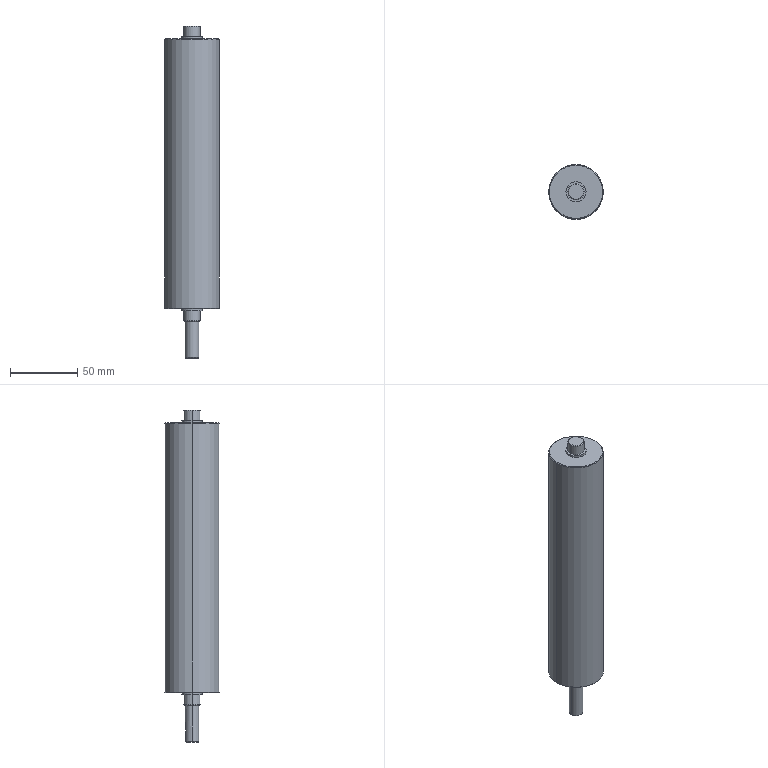Part | SolidWorks | features ICE 6, Chamfer 1, Extrusion 1, Fillet 1 | 1 solid | 35 faces | box 40.5 x 40.5 x 246 mm | volume 261959 mm3 | cylinder 14 | cone 11 | plane 10 | commonest cylinder face diameters 12 x4 15 x4 3 x2 10 x2 40.5 x2
STEP:
#1=CARTESIAN_POINT('',(5.5,0.,109.5));
#2=VERTEX_POINT('',#1);
#3=CARTESIAN_POINT('',(-5.5,0.,109.5));
#4=VERTEX_POINT('',#3);
#5=CARTESIAN_POINT('',(0.,0.,109.5));
#6=DIRECTION('',(0.,0.,1.));
#7=DIRECTION('',(1.,0.,0.));
#8=AXIS2_PLACEMENT_3D('',#5,#6,#7);
#9=CIRCLE('',#8,5.5);
#10=EDGE_CURVE('',#2,#4,#9,.T.);
#11=ORIENTED_EDGE('',*,*,#10,.F.);
#12=CARTESIAN_POINT('',(6.,0.,109.));
#13=VERTEX_POINT('',#12);
#14=CARTESIAN_POINT('',(5.5,0.,109.5));
#15=DIRECTION('',(0.7071,0.,-0.7071));
#16=VECTOR('',#15,1000.);
#17=LINE('',#14,#16);
#18=EDGE_CURVE('',#2,#13,#17,.T.);
#19=ORIENTED_EDGE('',*,*,#18,.T.);
#20=CARTESIAN_POINT('',(-6.,0.,109.));
#21=VERTEX_POINT('',#20);
#22=CARTESIAN_POINT('',(0.,0.,109.));
#23=DIRECTION('',(0.,0.,-1.));
#24=DIRECTION('',(1.,0.,0.));
#25=AXIS2_PLACEMENT_3D('',#22,#23,#24);
#26=CIRCLE('',#25,6.);
#27=EDGE_CURVE('',#21,#13,#26,.T.);
#28=ORIENTED_EDGE('',*,*,#27,.F.);
#29=CARTESIAN_POINT('',(-5.5,0.,109.5));
#30=DIRECTION('',(-0.7071,0.,-0.7071));
#31=VECTOR('',#30,1000.);
#32=LINE('',#29,#31);
#33=EDGE_CURVE('',#4,#21,#32,.T.);
#34=ORIENTED_EDGE('',*,*,#33,.F.);
#35=EDGE_LOOP('',(#11,#19,#28,#34));
#36=FACE_OUTER_BOUND('',#35,.T.);
#37=CARTESIAN_POINT('',(0.,0.,109.5));
#38=DIRECTION('',(0.,0.,-1.));
#39=DIRECTION('',(-1.,0.,0.));
#40=AXIS2_PLACEMENT_3D('',#37,#38,#39);
#41=CONICAL_SURFACE('',#40,5.5,0.7854);
#42=ADVANCED_FACE('',(#36),#41,.T.);
#43=CARTESIAN_POINT('',(19.75,0.,100.));
#44=VERTEX_POINT('',#43);
#45=CARTESIAN_POINT('',(-19.75,0.,100.));
#46=VERTEX_POINT('',#45);
#47=CARTESIAN_POINT('',(0.,0.,100.));
#48=DIRECTION('',(0.,0.,1.));
#49=DIRECTION('',(1.,0.,0.));
#50=AXIS2_PLACEMENT_3D('',#47,#48,#49);
#51=CIRCLE('',#50,19.75);
#52=EDGE_CURVE('',#44,#46,#51,.T.);
#53=ORIENTED_EDGE('',*,*,#52,.F.);
#54=CARTESIAN_POINT('',(20.25,0.,99.5));
#55=VERTEX_POINT('',#54);
#56=CARTESIAN_POINT('',(19.75,0.,100.));
#57=DIRECTION('',(0.7071,0.,-0.7071));
#58=VECTOR('',#57,1000.);
#59=LINE('',#56,#58);
#60=EDGE_CURVE('',#44,#55,#59,.T.);
#61=ORIENTED_EDGE('',*,*,#60,.T.);
#62=CARTESIAN_POINT('',(-20.25,0.,99.5));
#63=VERTEX_POINT('',#62);
#64=CARTESIAN_POINT('',(0.,0.,99.5));
#65=DIRECTION('',(0.,0.,-1.));
#66=DIRECTION('',(1.,0.,0.));
#67=AXIS2_PLACEMENT_3D('',#64,#65,#66);
#68=CIRCLE('',#67,20.25);
#69=EDGE_CURVE('',#63,#55,#68,.T.);
#70=ORIENTED_EDGE('',*,*,#69,.F.);
#71=CARTESIAN_POINT('',(-19.75,0.,100.));
#72=DIRECTION('',(-0.7071,0.,-0.7071));
#73=VECTOR('',#72,1000.);
#74=LINE('',#71,#73);
#75=EDGE_CURVE('',#46,#63,#74,.T.);
#76=ORIENTED_EDGE('',*,*,#75,.F.);
#77=EDGE_LOOP('',(#53,#61,#70,#76));
#78=FACE_OUTER_BOUND('',#77,.T.);
#79=CARTESIAN_POINT('',(0.,0.,100.));
#80=DIRECTION('',(0.,0.,-1.));
#81=DIRECTION('',(-1.,0.,0.));
#82=AXIS2_PLACEMENT_3D('',#79,#80,#81);
#83=CONICAL_SURFACE('',#82,19.75,0.7854);
#84=ADVANCED_FACE('',(#78),#83,.T.);
#85=CARTESIAN_POINT('',(-19.75,0.,-100.));
#86=VERTEX_POINT('',#85);
#87=CARTESIAN_POINT('',(19.75,0.,-100.));
#88=VERTEX_POINT('',#87);
#89=CARTESIAN_POINT('',(0.,0.,-100.));
#90=DIRECTION('',(0.,0.,-1.));
#91=DIRECTION('',(1.,0.,0.));
#92=AXIS2_PLACEMENT_3D('',#89,#90,#91);
#93=CIRCLE('',#92,19.75);
#94=EDGE_CURVE('',#86,#88,#93,.T.);
#95=ORIENTED_EDGE('',*,*,#94,.F.);
#96=CARTESIAN_POINT('',(-20.25,0.,-99.5));
#97=VERTEX_POINT('',#96);
#98=CARTESIAN_POINT('',(-20.25,0.,-99.5));
#99=DIRECTION('',(-0.7071,0.,0.7071));
#100=VECTOR('',#99,1000.);
#101=LINE('',#98,#100);
#102=EDGE_CURVE('',#86,#97,#101,.T.);
#103=ORIENTED_EDGE('',*,*,#102,.T.);
#104=CARTESIAN_POINT('',(20.25,0.,-99.5));
#105=VERTEX_POINT('',#104);
#106=CARTESIAN_POINT('',(0.,0.,-99.5));
#107=DIRECTION('',(0.,0.,1.));
#108=DIRECTION('',(1.,0.,0.));
#109=AXIS2_PLACEMENT_3D('',#106,#107,#108);
#110=CIRCLE('',#109,20.25);
#111=EDGE_CURVE('',#105,#97,#110,.T.);
#112=ORIENTED_EDGE('',*,*,#111,.F.);
#113=CARTESIAN_POINT('',(20.25,0.,-99.5));
#114=DIRECTION('',(0.7071,0.,0.7071));
#115=VECTOR('',#114,1000.);
#116=LINE('',#113,#115);
#117=EDGE_CURVE('',#88,#105,#116,.T.);
#118=ORIENTED_EDGE('',*,*,#117,.F.);
#119=EDGE_LOOP('',(#95,#103,#112,#118));
#120=FACE_OUTER_BOUND('',#119,.T.);
#121=CARTESIAN_POINT('',(0.,0.,-99.5));
#122=DIRECTION('',(0.,0.,1.));
#123=DIRECTION('',(1.,0.,0.));
#124=AXIS2_PLACEMENT_3D('',#121,#122,#123);
#125=CONICAL_SURFACE('',#124,20.25,0.7854);
#126=ADVANCED_FACE('',(#120),#125,.T.);
#127=CARTESIAN_POINT('',(-4.5,0.,-136.5));
#128=VERTEX_POINT('',#127);
#129=CARTESIAN_POINT('',(-1.5,4.243,-136.5));
#130=VERTEX_POINT('',#129);
#131=CARTESIAN_POINT('',(0.,0.,-136.5));
#132=DIRECTION('',(0.,0.,-1.));
#133=DIRECTION('',(-1.,0.,0.));
#134=AXIS2_PLACEMENT_3D('',#131,#132,#133);
#135=CIRCLE('',#134,4.5);
#136=EDGE_CURVE('',#128,#130,#135,.T.);
#137=ORIENTED_EDGE('',*,*,#136,.F.);
#138=CARTESIAN_POINT('',(-5.,0.,-136.));
#139=VERTEX_POINT('',#138);
#140=CARTESIAN_POINT('',(-4.5,0.,-136.5));
#141=DIRECTION('',(-0.7071,0.,0.7071));
#142=VECTOR('',#141,1000.);
#143=LINE('',#140,#142);
#144=EDGE_CURVE('',#128,#139,#143,.T.);
#145=ORIENTED_EDGE('',*,*,#144,.T.);
#146=CARTESIAN_POINT('',(-1.5,4.77,-136.));
#147=VERTEX_POINT('',#146);
#148=CARTESIAN_POINT('',(0.,0.,-136.));
#149=DIRECTION('',(0.,0.,1.));
#150=DIRECTION('',(-1.,0.,0.));
#151=AXIS2_PLACEMENT_3D('',#148,#149,#150);
#152=CIRCLE('',#151,5.);
#153=EDGE_CURVE('',#147,#139,#152,.T.);
#154=ORIENTED_EDGE('',*,*,#153,.F.);
#155=CARTESIAN_POINT('',(-1.5,4.243,-136.5));
#156=CARTESIAN_POINT('',(-1.5,4.419,-136.334));
#157=CARTESIAN_POINT('',(-1.5,4.594,-136.167));
#158=CARTESIAN_POINT('',(-1.5,4.77,-136.));
#159=B_SPLINE_CURVE_WITH_KNOTS('',3,(#155,#156,#157,#158),.UNSPECIFIED.,.F.,.F.,(4,4),(0.004011,0.004736),.UNSPECIFIED.);
#160=EDGE_CURVE('',#130,#147,#159,.T.);
#161=ORIENTED_EDGE('',*,*,#160,.F.);
#162=EDGE_LOOP('',(#137,#145,#154,#161));
#163=FACE_OUTER_BOUND('',#162,.T.);
#164=CARTESIAN_POINT('',(0.,0.,-136.5));
#165=DIRECTION('',(0.,0.,1.));
#166=DIRECTION('',(1.,0.,0.));
#167=AXIS2_PLACEMENT_3D('',#164,#165,#166);
#168=CONICAL_SURFACE('',#167,4.5,0.7854);
#169=ADVANCED_FACE('',(#163),#168,.T.);
#170=ORIENTED_EDGE('',*,*,#144,.F.);
#171=CARTESIAN_POINT('',(4.5,0.,-136.5));
#172=VERTEX_POINT('',#171);
#173=CARTESIAN_POINT('',(0.,0.,-136.5));
#174=DIRECTION('',(0.,0.,-1.));
#175=DIRECTION('',(-1.,0.,0.));
#176=AXIS2_PLACEMENT_3D('',#173,#174,#175);
#177=CIRCLE('',#176,4.5);
#178=EDGE_CURVE('',#172,#128,#177,.T.);
#179=ORIENTED_EDGE('',*,*,#178,.F.);
#180=CARTESIAN_POINT('',(5.,0.,-136.));
#181=VERTEX_POINT('',#180);
#182=CARTESIAN_POINT('',(4.5,0.,-136.5));
#183=DIRECTION('',(0.7071,0.,0.7071));
#184=VECTOR('',#183,1000.);
#185=LINE('',#182,#184);
#186=EDGE_CURVE('',#172,#181,#185,.T.);
#187=ORIENTED_EDGE('',*,*,#186,.T.);
#188=CARTESIAN_POINT('',(0.,0.,-136.));
#189=DIRECTION('',(0.,0.,1.));
#190=DIRECTION('',(-1.,0.,0.));
#191=AXIS2_PLACEMENT_3D('',#188,#189,#190);
#192=CIRCLE('',#191,5.);
#193=EDGE_CURVE('',#139,#181,#192,.T.);
#194=ORIENTED_EDGE('',*,*,#193,.F.);
#195=EDGE_LOOP('',(#170,#179,#187,#194));
#196=FACE_OUTER_BOUND('',#195,.T.);
#197=CARTESIAN_POINT('',(0.,0.,-136.5));
#198=DIRECTION('',(0.,0.,1.));
#199=DIRECTION('',(1.,0.,0.));
#200=AXIS2_PLACEMENT_3D('',#197,#198,#199);
#201=CONICAL_SURFACE('',#200,4.5,0.7854);
#202=ADVANCED_FACE('',(#196),#201,.T.);
#203=CARTESIAN_POINT('',(-5.5,0.,-109.5));
#204=VERTEX_POINT('',#203);
#205=CARTESIAN_POINT('',(5.5,0.,-109.5));
#206=VERTEX_POINT('',#205);
#207=CARTESIAN_POINT('',(0.,0.,-109.5));
#208=DIRECTION('',(0.,0.,-1.));
#209=DIRECTION('',(-1.,0.,0.));
#210=AXIS2_PLACEMENT_3D('',#207,#208,#209);
#211=CIRCLE('',#210,5.5);
#212=EDGE_CURVE('',#204,#206,#211,.T.);
#213=ORIENTED_EDGE('',*,*,#212,.F.);
#214=CARTESIAN_POINT('',(-6.,0.,-109.));
#215=VERTEX_POINT('',#214);
#216=CARTESIAN_POINT('',(-5.5,0.,-109.5));
#217=DIRECTION('',(-0.7071,0.,0.7071));
#218=VECTOR('',#217,1000.);
#219=LINE('',#216,#218);
#220=EDGE_CURVE('',#204,#215,#219,.T.);
#221=ORIENTED_EDGE('',*,*,#220,.T.);
#222=CARTESIAN_POINT('',(6.,0.,-109.));
#223=VERTEX_POINT('',#222);
#224=CARTESIAN_POINT('',(0.,0.,-109.));
#225=DIRECTION('',(0.,0.,1.));
#226=DIRECTION('',(-1.,0.,0.));
#227=AXIS2_PLACEMENT_3D('',#224,#225,#226);
#228=CIRCLE('',#227,6.);
#229=EDGE_CURVE('',#223,#215,#228,.T.);
#230=ORIENTED_EDGE('',*,*,#229,.F.);
#231=CARTESIAN_POINT('',(5.5,0.,-109.5));
#232=DIRECTION('',(0.7071,0.,0.7071));
#233=VECTOR('',#232,1000.);
#234=LINE('',#231,#233);
#235=EDGE_CURVE('',#206,#223,#234,.T.);
#236=ORIENTED_EDGE('',*,*,#235,.F.);
#237=EDGE_LOOP('',(#213,#221,#230,#236));
#238=FACE_OUTER_BOUND('',#237,.T.);
#239=CARTESIAN_POINT('',(0.,0.,-109.5));
#240=DIRECTION('',(0.,0.,1.));
#241=DIRECTION('',(1.,0.,0.));
#242=AXIS2_PLACEMENT_3D('',#239,#240,#241);
#243=CONICAL_SURFACE('',#242,5.5,0.7854);
#244=ADVANCED_FACE('',(#238),#243,.T.);
#245=ORIENTED_EDGE('',*,*,#153,.T.);
#246=CARTESIAN_POINT('',(-5.,0.,-109.5));
#247=VERTEX_POINT('',#246);
#248=CARTESIAN_POINT('',(-5.,0.,-136.5));
#249=DIRECTION('',(0.,0.,1.));
#250=VECTOR('',#249,1000.);
#251=LINE('',#248,#250);
#252=EDGE_CURVE('',#139,#247,#251,.T.);
#253=ORIENTED_EDGE('',*,*,#252,.T.);
#254=CARTESIAN_POINT('',(5.,0.,-109.5));
#255=VERTEX_POINT('',#254);
#256=CARTESIAN_POINT('',(0.,0.,-109.5));
#257=DIRECTION('',(0.,0.,-1.));
#258=DIRECTION('',(-1.,0.,0.));
#259=AXIS2_PLACEMENT_3D('',#256,#257,#258);
#260=CIRCLE('',#259,5.);
#261=EDGE_CURVE('',#247,#255,#260,.T.);
#262=ORIENTED_EDGE('',*,*,#261,.T.);
#263=CARTESIAN_POINT('',(5.,0.,-136.5));
#264=DIRECTION('',(0.,0.,1.));
#265=VECTOR('',#264,1000.);
#266=LINE('',#263,#265);
#267=EDGE_CURVE('',#181,#255,#266,.T.);
#268=ORIENTED_EDGE('',*,*,#267,.F.);
#269=CARTESIAN_POINT('',(1.5,4.77,-136.));
#270=VERTEX_POINT('',#269);
#271=CARTESIAN_POINT('',(0.,0.,-136.));
#272=DIRECTION('',(0.,0.,1.));
#273=DIRECTION('',(-1.,0.,0.));
#274=AXIS2_PLACEMENT_3D('',#271,#272,#273);
#275=CIRCLE('',#274,5.);
#276=EDGE_CURVE('',#181,#270,#275,.T.);
#277=ORIENTED_EDGE('',*,*,#276,.T.);
#278=CARTESIAN_POINT('',(1.5,4.77,-123.));
#279=VERTEX_POINT('',#278);
#280=CARTESIAN_POINT('',(1.5,4.77,-121.5));
#281=DIRECTION('',(0.,0.,-1.));
#282=VECTOR('',#281,1000.);
#283=LINE('',#280,#282);
#284=EDGE_CURVE('',#279,#270,#283,.T.);
#285=ORIENTED_EDGE('',*,*,#284,.F.);
#286=CARTESIAN_POINT('',(0.,5.,-121.5));
#287=VERTEX_POINT('',#286);
#288=CARTESIAN_POINT('',(1.5,4.77,-123.));
#289=CARTESIAN_POINT('',(1.5,4.77,-122.9));
#290=CARTESIAN_POINT('',(1.49,4.773,-122.802));
#291=CARTESIAN_POINT('',(1.452,4.785,-122.61));
#292=CARTESIAN_POINT('',(1.423,4.793,-122.515));
#293=CARTESIAN_POINT('',(1.347,4.815,-122.333));
#294=CARTESIAN_POINT('',(1.301,4.828,-122.247));
#295=CARTESIAN_POINT('',(1.193,4.856,-122.085));
#296=CARTESIAN_POINT('',(1.13,4.871,-122.008));
#297=CARTESIAN_POINT('',(0.9236,4.916,-121.802));
#298=CARTESIAN_POINT('',(0.7574,4.946,-121.691));
#299=CARTESIAN_POINT('',(0.3971,4.988,-121.54));
#300=CARTESIAN_POINT('',(0.1993,5.,-121.5));
#301=CARTESIAN_POINT('',(0.,5.,-121.5));
#302=B_SPLINE_CURVE_WITH_KNOTS('',3,(#288,#289,#290,#291,#292,#293,#294,#295,#296,#297,#298,#299,#300,#301),.UNSPECIFIED.,.F.,.F.,(4,2,2,2,2,2,4),(0.,0.0002946,0.0005892,0.0008838,0.001178,0.001768,0.002357),.UNSPECIFIED.);
#303=EDGE_CURVE('',#279,#287,#302,.T.);
#304=ORIENTED_EDGE('',*,*,#303,.T.);
#305=CARTESIAN_POINT('',(-1.5,4.77,-123.));
#306=VERTEX_POINT('',#305);
#307=CARTESIAN_POINT('',(0.,5.,-121.5));
#308=CARTESIAN_POINT('',(-0.09966,5.,-121.5));
#309=CARTESIAN_POINT('',(-0.1975,4.997,-121.51));
#310=CARTESIAN_POINT('',(-0.3899,4.986,-121.548));
#311=CARTESIAN_POINT('',(-0.4855,4.977,-121.577));
#312=CARTESIAN_POINT('',(-0.6668,4.956,-121.653));
#313=CARTESIAN_POINT('',(-0.7527,4.944,-121.699));
#314=CARTESIAN_POINT('',(-0.9153,4.916,-121.808));
#315=CARTESIAN_POINT('',(-0.9918,4.901,-121.87));
#316=CARTESIAN_POINT('',(-1.198,4.856,-122.077));
#317=CARTESIAN_POINT('',(-1.309,4.826,-122.243));
#318=CARTESIAN_POINT('',(-1.46,4.783,-122.603));
#319=CARTESIAN_POINT('',(-1.5,4.77,-122.801));
#320=CARTESIAN_POINT('',(-1.5,4.77,-123.));
#321=B_SPLINE_CURVE_WITH_KNOTS('',3,(#307,#308,#309,#310,#311,#312,#313,#314,#315,#316,#317,#318,#319,#320),.UNSPECIFIED.,.F.,.F.,(4,2,2,2,2,2,4),(0.,0.0002946,0.0005892,0.0008839,0.001178,0.001768,0.002357),.UNSPECIFIED.);
#322=EDGE_CURVE('',#287,#306,#321,.T.);
#323=ORIENTED_EDGE('',*,*,#322,.T.);
#324=CARTESIAN_POINT('',(-1.5,4.77,-121.5));
#325=DIRECTION('',(0.,0.,-1.));
#326=VECTOR('',#325,1000.);
#327=LINE('',#324,#326);
#328=EDGE_CURVE('',#306,#147,#327,.T.);
#329=ORIENTED_EDGE('',*,*,#328,.T.);
#330=EDGE_LOOP('',(#245,#253,#262,#268,#277,#285,#304,#323,#329));
#331=FACE_OUTER_BOUND('',#330,.T.);
#332=CARTESIAN_POINT('',(0.,0.,-136.5));
#333=DIRECTION('',(0.,0.,1.));
#334=DIRECTION('',(1.,0.,0.));
#335=AXIS2_PLACEMENT_3D('',#332,#333,#334);
#336=CYLINDRICAL_SURFACE('',#335,5.);
#337=ADVANCED_FACE('',(#331),#336,.T.);
#338=ORIENTED_EDGE('',*,*,#229,.T.);
#339=CARTESIAN_POINT('',(-6.,0.,-101.5));
#340=VERTEX_POINT('',#339);
#341=CARTESIAN_POINT('',(-6.,0.,-109.5));
#342=DIRECTION('',(0.,0.,1.));
#343=VECTOR('',#342,1000.);
#344=LINE('',#341,#343);
#345=EDGE_CURVE('',#215,#340,#344,.T.);
#346=ORIENTED_EDGE('',*,*,#345,.T.);
#347=CARTESIAN_POINT('',(6.,0.,-101.5));
#348=VERTEX_POINT('',#347);
#349=CARTESIAN_POINT('',(0.,0.,-101.5));
#350=DIRECTION('',(0.,0.,-1.));
#351=DIRECTION('',(-1.,0.,0.));
#352=AXIS2_PLACEMENT_3D('',#349,#350,#351);
#353=CIRCLE('',#352,6.);
#354=EDGE_CURVE('',#340,#348,#353,.T.);
#355=ORIENTED_EDGE('',*,*,#354,.T.);
#356=CARTESIAN_POINT('',(6.,0.,-109.5));
#357=DIRECTION('',(0.,0.,1.));
#358=VECTOR('',#357,1000.);
#359=LINE('',#356,#358);
#360=EDGE_CURVE('',#223,#348,#359,.T.);
#361=ORIENTED_EDGE('',*,*,#360,.F.);
#362=EDGE_LOOP('',(#338,#346,#355,#361));
#363=FACE_OUTER_BOUND('',#362,.T.);
#364=CARTESIAN_POINT('',(0.,0.,-109.5));
#365=DIRECTION('',(0.,0.,1.));
#366=DIRECTION('',(1.,0.,0.));
#367=AXIS2_PLACEMENT_3D('',#364,#365,#366);
#368=CYLINDRICAL_SURFACE('',#367,6.);
#369=ADVANCED_FACE('',(#363),#368,.T.);
#370=ORIENTED_EDGE('',*,*,#27,.T.);
#371=CARTESIAN_POINT('',(6.,0.,101.5));
#372=VERTEX_POINT('',#371);
#373=CARTESIAN_POINT('',(6.,0.,109.5));
#374=DIRECTION('',(0.,0.,-1.));
#375=VECTOR('',#374,1000.);
#376=LINE('',#373,#375);
#377=EDGE_CURVE('',#13,#372,#376,.T.);
#378=ORIENTED_EDGE('',*,*,#377,.T.);
#379=CARTESIAN_POINT('',(-6.,0.,101.5));
#380=VERTEX_POINT('',#379);
#381=CARTESIAN_POINT('',(0.,0.,101.5));
#382=DIRECTION('',(0.,0.,1.));
#383=DIRECTION('',(1.,0.,0.));
#384=AXIS2_PLACEMENT_3D('',#381,#382,#383);
#385=CIRCLE('',#384,6.);
#386=EDGE_CURVE('',#372,#380,#385,.T.);
#387=ORIENTED_EDGE('',*,*,#386,.T.);
#388=CARTESIAN_POINT('',(-6.,0.,109.5));
#389=DIRECTION('',(0.,0.,-1.));
#390=VECTOR('',#389,1000.);
#391=LINE('',#388,#390);
#392=EDGE_CURVE('',#21,#380,#391,.T.);
#393=ORIENTED_EDGE('',*,*,#392,.F.);
#394=EDGE_LOOP('',(#370,#378,#387,#393));
#395=FACE_OUTER_BOUND('',#394,.T.);
#396=CARTESIAN_POINT('',(0.,0.,109.5));
#397=DIRECTION('',(0.,0.,-1.));
#398=DIRECTION('',(-1.,0.,0.));
#399=AXIS2_PLACEMENT_3D('',#396,#397,#398);
#400=CYLINDRICAL_SURFACE('',#399,6.);
#401=ADVANCED_FACE('',(#395),#400,.T.);
#402=CARTESIAN_POINT('',(7.5,0.,101.5));
#403=VERTEX_POINT('',#402);
#404=CARTESIAN_POINT('',(-7.5,0.,101.5));
#405=VERTEX_POINT('',#404);
#406=CARTESIAN_POINT('',(0.,0.,101.5));
#407=DIRECTION('',(0.,0.,1.));
#408=DIRECTION('',(1.,0.,0.));
#409=AXIS2_PLACEMENT_3D('',#406,#407,#408);
#410=CIRCLE('',#409,7.5);
#411=EDGE_CURVE('',#403,#405,#410,.T.);
#412=ORIENTED_EDGE('',*,*,#411,.F.);
#413=CARTESIAN_POINT('',(7.5,0.,100.));
#414=VERTEX_POINT('',#413);
#415=CARTESIAN_POINT('',(7.5,0.,101.5));
#416=DIRECTION('',(0.,0.,-1.));
#417=VECTOR('',#416,1000.);
#418=LINE('',#415,#417);
#419=EDGE_CURVE('',#403,#414,#418,.T.);
#420=ORIENTED_EDGE('',*,*,#419,.T.);
#421=CARTESIAN_POINT('',(-7.5,0.,100.));
#422=VERTEX_POINT('',#421);
#423=CARTESIAN_POINT('',(0.,0.,100.));
#424=DIRECTION('',(0.,0.,1.));
#425=DIRECTION('',(1.,0.,0.));
#426=AXIS2_PLACEMENT_3D('',#423,#424,#425);
#427=CIRCLE('',#426,7.5);
#428=EDGE_CURVE('',#414,#422,#427,.T.);
#429=ORIENTED_EDGE('',*,*,#428,.T.);
#430=CARTESIAN_POINT('',(-7.5,0.,101.5));
#431=DIRECTION('',(0.,0.,-1.));
#432=VECTOR('',#431,1000.);
#433=LINE('',#430,#432);
#434=EDGE_CURVE('',#405,#422,#433,.T.);
#435=ORIENTED_EDGE('',*,*,#434,.F.);
#436=EDGE_LOOP('',(#412,#420,#429,#435));
#437=FACE_OUTER_BOUND('',#436,.T.);
#438=CARTESIAN_POINT('',(0.,0.,101.5));
#439=DIRECTION('',(0.,0.,-1.));
#440=DIRECTION('',(-1.,0.,0.));
#441=AXIS2_PLACEMENT_3D('',#438,#439,#440);
#442=CYLINDRICAL_SURFACE('',#441,7.5);
#443=ADVANCED_FACE('',(#437),#442,.T.);
#444=CARTESIAN_POINT('',(-7.5,0.,-101.5));
#445=VERTEX_POINT('',#444);
#446=CARTESIAN_POINT('',(7.5,0.,-101.5));
#447=VERTEX_POINT('',#446);
#448=CARTESIAN_POINT('',(0.,0.,-101.5));
#449=DIRECTION('',(0.,0.,-1.));
#450=DIRECTION('',(-1.,0.,0.));
#451=AXIS2_PLACEMENT_3D('',#448,#449,#450);
#452=CIRCLE('',#451,7.5);
#453=EDGE_CURVE('',#445,#447,#452,.T.);
#454=ORIENTED_EDGE('',*,*,#453,.F.);
#455=CARTESIAN_POINT('',(-7.5,0.,-100.));
#456=VERTEX_POINT('',#455);
#457=CARTESIAN_POINT('',(-7.5,0.,-101.5));
#458=DIRECTION('',(0.,0.,1.));
#459=VECTOR('',#458,1000.);
#460=LINE('',#457,#459);
#461=EDGE_CURVE('',#445,#456,#460,.T.);
#462=ORIENTED_EDGE('',*,*,#461,.T.);
#463=CARTESIAN_POINT('',(7.5,0.,-100.));
#464=VERTEX_POINT('',#463);
#465=CARTESIAN_POINT('',(0.,0.,-100.));
#466=DIRECTION('',(0.,0.,-1.));
#467=DIRECTION('',(-1.,0.,0.));
#468=AXIS2_PLACEMENT_3D('',#465,#466,#467);
#469=CIRCLE('',#468,7.5);
#470=EDGE_CURVE('',#456,#464,#469,.T.);
#471=ORIENTED_EDGE('',*,*,#470,.T.);
#472=CARTESIAN_POINT('',(7.5,0.,-101.5));
#473=DIRECTION('',(0.,0.,1.));
#474=VECTOR('',#473,1000.);
#475=LINE('',#472,#474);
#476=EDGE_CURVE('',#447,#464,#475,.T.);
#477=ORIENTED_EDGE('',*,*,#476,.F.);
#478=EDGE_LOOP('',(#454,#462,#471,#477));
#479=FACE_OUTER_BOUND('',#478,.T.);
#480=CARTESIAN_POINT('',(0.,0.,-101.5));
#481=DIRECTION('',(0.,0.,1.));
#482=DIRECTION('',(1.,0.,0.));
#483=AXIS2_PLACEMENT_3D('',#480,#481,#482);
#484=CYLINDRICAL_SURFACE('',#483,7.5);
#485=ADVANCED_FACE('',(#479),#484,.T.);
#486=ORIENTED_EDGE('',*,*,#69,.T.);
#487=CARTESIAN_POINT('',(20.25,0.,100.));
#488=DIRECTION('',(0.,0.,-1.));
#489=VECTOR('',#488,1000.);
#490=LINE('',#487,#489);
#491=EDGE_CURVE('',#55,#105,#490,.T.);
#492=ORIENTED_EDGE('',*,*,#491,.T.);
#493=ORIENTED_EDGE('',*,*,#111,.T.);
#494=CARTESIAN_POINT('',(-20.25,0.,100.));
#495=DIRECTION('',(0.,0.,-1.));
#496=VECTOR('',#495,1000.);
#497=LINE('',#494,#496);
#498=EDGE_CURVE('',#63,#97,#497,.T.);
#499=ORIENTED_EDGE('',*,*,#498,.F.);
#500=EDGE_LOOP('',(#486,#492,#493,#499));
#501=FACE_OUTER_BOUND('',#500,.T.);
#502=CARTESIAN_POINT('',(0.,0.,100.));
#503=DIRECTION('',(0.,0.,-1.));
#504=DIRECTION('',(-1.,0.,0.));
#505=AXIS2_PLACEMENT_3D('',#502,#503,#504);
#506=CYLINDRICAL_SURFACE('',#505,20.25);
#507=ADVANCED_FACE('',(#501),#506,.T.);
#508=ORIENTED_EDGE('',*,*,#491,.F.);
#509=CARTESIAN_POINT('',(0.,0.,99.5));
#510=DIRECTION('',(0.,0.,-1.));
#511=DIRECTION('',(1.,0.,0.));
#512=AXIS2_PLACEMENT_3D('',#509,#510,#511);
#513=CIRCLE('',#512,20.25);
#514=EDGE_CURVE('',#55,#63,#513,.T.);
#515=ORIENTED_EDGE('',*,*,#514,.T.);
#516=ORIENTED_EDGE('',*,*,#498,.T.);
#517=CARTESIAN_POINT('',(0.,0.,-99.5));
#518=DIRECTION('',(0.,0.,1.));
#519=DIRECTION('',(1.,0.,0.));
#520=AXIS2_PLACEMENT_3D('',#517,#518,#519);
#521=CIRCLE('',#520,20.25);
#522=EDGE_CURVE('',#97,#105,#521,.T.);
#523=ORIENTED_EDGE('',*,*,#522,.T.);
#524=EDGE_LOOP('',(#508,#515,#516,#523));
#525=FACE_OUTER_BOUND('',#524,.T.);
#526=CARTESIAN_POINT('',(0.,0.,100.));
#527=DIRECTION('',(0.,0.,-1.));
#528=DIRECTION('',(-1.,0.,0.));
#529=AXIS2_PLACEMENT_3D('',#526,#527,#528);
#530=CYLINDRICAL_SURFACE('',#529,20.25);
#531=ADVANCED_FACE('',(#525),#530,.T.);
#532=CARTESIAN_POINT('',(0.,0.,100.));
#533=DIRECTION('',(0.,0.,1.));
#534=DIRECTION('',(1.,0.,0.));
#535=AXIS2_PLACEMENT_3D('',#532,#533,#534);
#536=CIRCLE('',#535,19.75);
#537=EDGE_CURVE('',#46,#44,#536,.T.);
#538=ORIENTED_EDGE('',*,*,#537,.T.);
#539=ORIENTED_EDGE('',*,*,#52,.T.);
#540=EDGE_LOOP('',(#538,#539));
#541=FACE_OUTER_BOUND('',#540,.T.);
#542=CARTESIAN_POINT('',(0.,0.,100.));
#543=DIRECTION('',(0.,0.,1.));
#544=DIRECTION('',(1.,0.,0.));
#545=AXIS2_PLACEMENT_3D('',#542,#543,#544);
#546=CIRCLE('',#545,7.5);
#547=EDGE_CURVE('',#422,#414,#546,.T.);
#548=ORIENTED_EDGE('',*,*,#547,.F.);
#549=ORIENTED_EDGE('',*,*,#428,.F.);
#550=EDGE_LOOP('',(#548,#549));
#551=FACE_BOUND('',#550,.T.);
#552=CARTESIAN_POINT('',(0.,0.,100.));
#553=DIRECTION('',(0.,0.,1.));
#554=DIRECTION('',(1.,0.,0.));
#555=AXIS2_PLACEMENT_3D('',#552,#553,#554);
#556=PLANE('',#555);
#557=ADVANCED_FACE('',(#541,#551),#556,.T.);
#558=CARTESIAN_POINT('',(0.,0.,-100.));
#559=DIRECTION('',(0.,0.,-1.));
#560=DIRECTION('',(1.,0.,0.));
#561=AXIS2_PLACEMENT_3D('',#558,#559,#560);
#562=CIRCLE('',#561,19.75);
#563=EDGE_CURVE('',#88,#86,#562,.T.);
#564=ORIENTED_EDGE('',*,*,#563,.T.);
#565=ORIENTED_EDGE('',*,*,#94,.T.);
#566=EDGE_LOOP('',(#564,#565));
#567=FACE_OUTER_BOUND('',#566,.T.);
#568=CARTESIAN_POINT('',(0.,0.,-100.));
#569=DIRECTION('',(0.,0.,-1.));
#570=DIRECTION('',(-1.,0.,0.));
#571=AXIS2_PLACEMENT_3D('',#568,#569,#570);
#572=CIRCLE('',#571,7.5);
#573=EDGE_CURVE('',#464,#456,#572,.T.);
#574=ORIENTED_EDGE('',*,*,#573,.F.);
#575=ORIENTED_EDGE('',*,*,#470,.F.);
#576=EDGE_LOOP('',(#574,#575));
#577=FACE_BOUND('',#576,.T.);
#578=CARTESIAN_POINT('',(0.,0.,-100.));
#579=DIRECTION('',(0.,0.,1.));
#580=DIRECTION('',(1.,0.,0.));
#581=AXIS2_PLACEMENT_3D('',#578,#579,#580);
#582=PLANE('',#581);
#583=ADVANCED_FACE('',(#567,#577),#582,.F.);
#584=ORIENTED_EDGE('',*,*,#461,.F.);
#585=CARTESIAN_POINT('',(0.,0.,-101.5));
#586=DIRECTION('',(0.,0.,-1.));
#587=DIRECTION('',(-1.,0.,0.));
#588=AXIS2_PLACEMENT_3D('',#585,#586,#587);
#589=CIRCLE('',#588,7.5);
#590=EDGE_CURVE('',#447,#445,#589,.T.);
#591=ORIENTED_EDGE('',*,*,#590,.F.);
#592=ORIENTED_EDGE('',*,*,#476,.T.);
#593=ORIENTED_EDGE('',*,*,#573,.T.);
#594=EDGE_LOOP('',(#584,#591,#592,#593));
#595=FACE_OUTER_BOUND('',#594,.T.);
#596=CARTESIAN_POINT('',(0.,0.,-101.5));
#597=DIRECTION('',(0.,0.,1.));
#598=DIRECTION('',(1.,0.,0.));
#599=AXIS2_PLACEMENT_3D('',#596,#597,#598);
#600=CYLINDRICAL_SURFACE('',#599,7.5);
#601=ADVANCED_FACE('',(#595),#600,.T.);
#602=CARTESIAN_POINT('',(0.,0.,-101.5));
#603=DIRECTION('',(0.,0.,-1.));
#604=DIRECTION('',(-1.,0.,0.));
#605=AXIS2_PLACEMENT_3D('',#602,#603,#604);
#606=CIRCLE('',#605,6.);
#607=EDGE_CURVE('',#348,#340,#606,.T.);
#608=ORIENTED_EDGE('',*,*,#607,.F.);
#609=ORIENTED_EDGE('',*,*,#354,.F.);
#610=EDGE_LOOP('',(#608,#609));
#611=FACE_BOUND('',#610,.T.);
#612=ORIENTED_EDGE('',*,*,#590,.T.);
#613=ORIENTED_EDGE('',*,*,#453,.T.);
#614=EDGE_LOOP('',(#612,#613));
#615=FACE_OUTER_BOUND('',#614,.T.);
#616=CARTESIAN_POINT('',(0.,0.,-101.5));
#617=DIRECTION('',(0.,0.,-1.));
#618=DIRECTION('',(-1.,0.,0.));
#619=AXIS2_PLACEMENT_3D('',#616,#617,#618);
#620=PLANE('',#619);
#621=ADVANCED_FACE('',(#611,#615),#620,.T.);
#622=ORIENTED_EDGE('',*,*,#419,.F.);
#623=CARTESIAN_POINT('',(0.,0.,101.5));
#624=DIRECTION('',(0.,0.,1.));
#625=DIRECTION('',(1.,0.,0.));
#626=AXIS2_PLACEMENT_3D('',#623,#624,#625);
#627=CIRCLE('',#626,7.5);
#628=EDGE_CURVE('',#405,#403,#627,.T.);
#629=ORIENTED_EDGE('',*,*,#628,.F.);
#630=ORIENTED_EDGE('',*,*,#434,.T.);
#631=ORIENTED_EDGE('',*,*,#547,.T.);
#632=EDGE_LOOP('',(#622,#629,#630,#631));
#633=FACE_OUTER_BOUND('',#632,.T.);
#634=CARTESIAN_POINT('',(0.,0.,101.5));
#635=DIRECTION('',(0.,0.,-1.));
#636=DIRECTION('',(-1.,0.,0.));
#637=AXIS2_PLACEMENT_3D('',#634,#635,#636);
#638=CYLINDRICAL_SURFACE('',#637,7.5);
#639=ADVANCED_FACE('',(#633),#638,.T.);
#640=CARTESIAN_POINT('',(0.,0.,101.5));
#641=DIRECTION('',(0.,0.,1.));
#642=DIRECTION('',(1.,0.,0.));
#643=AXIS2_PLACEMENT_3D('',#640,#641,#642);
#644=CIRCLE('',#643,6.);
#645=EDGE_CURVE('',#380,#372,#644,.T.);
#646=ORIENTED_EDGE('',*,*,#645,.F.);
#647=ORIENTED_EDGE('',*,*,#386,.F.);
#648=EDGE_LOOP('',(#646,#647));
#649=FACE_BOUND('',#648,.T.);
#650=ORIENTED_EDGE('',*,*,#628,.T.);
#651=ORIENTED_EDGE('',*,*,#411,.T.);
#652=EDGE_LOOP('',(#650,#651));
#653=FACE_OUTER_BOUND('',#652,.T.);
#654=CARTESIAN_POINT('',(0.,0.,101.5));
#655=DIRECTION('',(0.,0.,1.));
#656=DIRECTION('',(1.,0.,0.));
#657=AXIS2_PLACEMENT_3D('',#654,#655,#656);
#658=PLANE('',#657);
#659=ADVANCED_FACE('',(#649,#653),#658,.T.);
#660=ORIENTED_EDGE('',*,*,#377,.F.);
#661=CARTESIAN_POINT('',(0.,0.,109.));
#662=DIRECTION('',(0.,0.,-1.));
#663=DIRECTION('',(1.,0.,0.));
#664=AXIS2_PLACEMENT_3D('',#661,#662,#663);
#665=CIRCLE('',#664,6.);
#666=EDGE_CURVE('',#13,#21,#665,.T.);
#667=ORIENTED_EDGE('',*,*,#666,.T.);
#668=ORIENTED_EDGE('',*,*,#392,.T.);
#669=ORIENTED_EDGE('',*,*,#645,.T.);
#670=EDGE_LOOP('',(#660,#667,#668,#669));
#671=FACE_OUTER_BOUND('',#670,.T.);
#672=CARTESIAN_POINT('',(0.,0.,109.5));
#673=DIRECTION('',(0.,0.,-1.));
#674=DIRECTION('',(-1.,0.,0.));
#675=AXIS2_PLACEMENT_3D('',#672,#673,#674);
#676=CYLINDRICAL_SURFACE('',#675,6.);
#677=ADVANCED_FACE('',(#671),#676,.T.);
#678=CARTESIAN_POINT('',(0.,0.,109.5));
#679=DIRECTION('',(0.,0.,1.));
#680=DIRECTION('',(1.,0.,0.));
#681=AXIS2_PLACEMENT_3D('',#678,#679,#680);
#682=CIRCLE('',#681,5.5);
#683=EDGE_CURVE('',#4,#2,#682,.T.);
#684=ORIENTED_EDGE('',*,*,#683,.T.);
#685=ORIENTED_EDGE('',*,*,#10,.T.);
#686=EDGE_LOOP('',(#684,#685));
#687=FACE_OUTER_BOUND('',#686,.T.);
#688=CARTESIAN_POINT('',(0.,0.,109.5));
#689=DIRECTION('',(0.,0.,1.));
#690=DIRECTION('',(1.,0.,0.));
#691=AXIS2_PLACEMENT_3D('',#688,#689,#690);
#692=PLANE('',#691);
#693=ADVANCED_FACE('',(#687),#692,.T.);
#694=ORIENTED_EDGE('',*,*,#345,.F.);
#695=CARTESIAN_POINT('',(0.,0.,-109.));
#696=DIRECTION('',(0.,0.,1.));
#697=DIRECTION('',(-1.,0.,0.));
#698=AXIS2_PLACEMENT_3D('',#695,#696,#697);
#699=CIRCLE('',#698,6.);
#700=EDGE_CURVE('',#215,#223,#699,.T.);
#701=ORIENTED_EDGE('',*,*,#700,.T.);
#702=ORIENTED_EDGE('',*,*,#360,.T.);
#703=ORIENTED_EDGE('',*,*,#607,.T.);
#704=EDGE_LOOP('',(#694,#701,#702,#703));
#705=FACE_OUTER_BOUND('',#704,.T.);
#706=CARTESIAN_POINT('',(0.,0.,-109.5));
#707=DIRECTION('',(0.,0.,1.));
#708=DIRECTION('',(1.,0.,0.));
#709=AXIS2_PLACEMENT_3D('',#706,#707,#708);
#710=CYLINDRICAL_SURFACE('',#709,6.);
#711=ADVANCED_FACE('',(#705),#710,.T.);
#712=CARTESIAN_POINT('',(0.,0.,-109.5));
#713=DIRECTION('',(0.,0.,-1.));
#714=DIRECTION('',(-1.,0.,0.));
#715=AXIS2_PLACEMENT_3D('',#712,#713,#714);
#716=CIRCLE('',#715,5.5);
#717=EDGE_CURVE('',#206,#204,#716,.T.);
#718=ORIENTED_EDGE('',*,*,#717,.T.);
#719=ORIENTED_EDGE('',*,*,#212,.T.);
#720=EDGE_LOOP('',(#718,#719));
#721=FACE_OUTER_BOUND('',#720,.T.);
#722=CARTESIAN_POINT('',(0.,0.,-109.5));
#723=DIRECTION('',(0.,0.,-1.));
#724=DIRECTION('',(-1.,0.,0.));
#725=AXIS2_PLACEMENT_3D('',#722,#723,#724);
#726=CIRCLE('',#725,5.);
#727=EDGE_CURVE('',#255,#247,#726,.T.);
#728=ORIENTED_EDGE('',*,*,#727,.F.);
#729=ORIENTED_EDGE('',*,*,#261,.F.);
#730=EDGE_LOOP('',(#728,#729));
#731=FACE_BOUND('',#730,.T.);
#732=CARTESIAN_POINT('',(0.,0.,-109.5));
#733=DIRECTION('',(0.,0.,-1.));
#734=DIRECTION('',(-1.,0.,0.));
#735=AXIS2_PLACEMENT_3D('',#732,#733,#734);
#736=PLANE('',#735);
#737=ADVANCED_FACE('',(#721,#731),#736,.T.);
#738=ORIENTED_EDGE('',*,*,#252,.F.);
#739=ORIENTED_EDGE('',*,*,#193,.T.);
#740=ORIENTED_EDGE('',*,*,#267,.T.);
#741=ORIENTED_EDGE('',*,*,#727,.T.);
#742=EDGE_LOOP('',(#738,#739,#740,#741));
#743=FACE_OUTER_BOUND('',#742,.T.);
#744=CARTESIAN_POINT('',(0.,0.,-136.5));
#745=DIRECTION('',(0.,0.,1.));
#746=DIRECTION('',(1.,0.,0.));
#747=AXIS2_PLACEMENT_3D('',#744,#745,#746);
#748=CYLINDRICAL_SURFACE('',#747,5.);
#749=ADVANCED_FACE('',(#743),#748,.T.);
#750=CARTESIAN_POINT('',(-1.5,2.5,-136.5));
#751=VERTEX_POINT('',#750);
#752=CARTESIAN_POINT('',(-1.5,2.5,-136.5));
#753=DIRECTION('',(0.,1.,0.));
#754=VECTOR('',#753,1000.);
#755=LINE('',#752,#754);
#756=EDGE_CURVE('',#751,#130,#755,.T.);
#757=ORIENTED_EDGE('',*,*,#756,.F.);
#758=CARTESIAN_POINT('',(1.5,2.5,-136.5));
#759=VERTEX_POINT('',#758);
#760=CARTESIAN_POINT('',(1.5,2.5,-136.5));
#761=DIRECTION('',(-1.,0.,0.));
#762=VECTOR('',#761,1000.);
#763=LINE('',#760,#762);
#764=EDGE_CURVE('',#759,#751,#763,.T.);
#765=ORIENTED_EDGE('',*,*,#764,.F.);
#766=CARTESIAN_POINT('',(1.5,4.243,-136.5));
#767=VERTEX_POINT('',#766);
#768=CARTESIAN_POINT('',(1.5,4.77,-136.5));
#769=DIRECTION('',(0.,-1.,0.));
#770=VECTOR('',#769,1000.);
#771=LINE('',#768,#770);
#772=EDGE_CURVE('',#767,#759,#771,.T.);
#773=ORIENTED_EDGE('',*,*,#772,.F.);
#774=CARTESIAN_POINT('',(0.,0.,-136.5));
#775=DIRECTION('',(0.,0.,-1.));
#776=DIRECTION('',(-1.,0.,0.));
#777=AXIS2_PLACEMENT_3D('',#774,#775,#776);
#778=CIRCLE('',#777,4.5);
#779=EDGE_CURVE('',#767,#172,#778,.T.);
#780=ORIENTED_EDGE('',*,*,#779,.T.);
#781=ORIENTED_EDGE('',*,*,#178,.T.);
#782=ORIENTED_EDGE('',*,*,#136,.T.);
#783=EDGE_LOOP('',(#757,#765,#773,#780,#781,#782));
#784=FACE_OUTER_BOUND('',#783,.T.);
#785=CARTESIAN_POINT('',(0.,0.,-136.5));
#786=DIRECTION('',(0.,0.,-1.));
#787=DIRECTION('',(-1.,0.,0.));
#788=AXIS2_PLACEMENT_3D('',#785,#786,#787);
#789=PLANE('',#788);
#790=ADVANCED_FACE('',(#784),#789,.T.);
#791=ORIENTED_EDGE('',*,*,#220,.F.);
#792=ORIENTED_EDGE('',*,*,#717,.F.);
#793=ORIENTED_EDGE('',*,*,#235,.T.);
#794=ORIENTED_EDGE('',*,*,#700,.F.);
#795=EDGE_LOOP('',(#791,#792,#793,#794));
#796=FACE_OUTER_BOUND('',#795,.T.);
#797=CARTESIAN_POINT('',(0.,0.,-109.5));
#798=DIRECTION('',(0.,0.,1.));
#799=DIRECTION('',(1.,0.,0.));
#800=AXIS2_PLACEMENT_3D('',#797,#798,#799);
#801=CONICAL_SURFACE('',#800,5.5,0.7854);
#802=ADVANCED_FACE('',(#796),#801,.T.);
#803=ORIENTED_EDGE('',*,*,#186,.F.);
#804=ORIENTED_EDGE('',*,*,#779,.F.);
#805=CARTESIAN_POINT('',(1.5,4.77,-136.));
#806=CARTESIAN_POINT('',(1.5,4.594,-136.167));
#807=CARTESIAN_POINT('',(1.5,4.419,-136.334));
#808=CARTESIAN_POINT('',(1.5,4.243,-136.5));
#809=B_SPLINE_CURVE_WITH_KNOTS('',3,(#805,#806,#807,#808),.UNSPECIFIED.,.F.,.F.,(4,4),(0.003975,0.004701),.UNSPECIFIED.);
#810=EDGE_CURVE('',#270,#767,#809,.T.);
#811=ORIENTED_EDGE('',*,*,#810,.F.);
#812=ORIENTED_EDGE('',*,*,#276,.F.);
#813=EDGE_LOOP('',(#803,#804,#811,#812));
#814=FACE_OUTER_BOUND('',#813,.T.);
#815=CARTESIAN_POINT('',(0.,0.,-136.5));
#816=DIRECTION('',(0.,0.,1.));
#817=DIRECTION('',(1.,0.,0.));
#818=AXIS2_PLACEMENT_3D('',#815,#816,#817);
#819=CONICAL_SURFACE('',#818,4.5,0.7854);
#820=ADVANCED_FACE('',(#814),#819,.T.);
#821=ORIENTED_EDGE('',*,*,#102,.F.);
#822=ORIENTED_EDGE('',*,*,#563,.F.);
#823=ORIENTED_EDGE('',*,*,#117,.T.);
#824=ORIENTED_EDGE('',*,*,#522,.F.);
#825=EDGE_LOOP('',(#821,#822,#823,#824));
#826=FACE_OUTER_BOUND('',#825,.T.);
#827=CARTESIAN_POINT('',(0.,0.,-99.5));
#828=DIRECTION('',(0.,0.,1.));
#829=DIRECTION('',(1.,0.,0.));
#830=AXIS2_PLACEMENT_3D('',#827,#828,#829);
#831=CONICAL_SURFACE('',#830,20.25,0.7854);
#832=ADVANCED_FACE('',(#826),#831,.T.);
#833=ORIENTED_EDGE('',*,*,#60,.F.);
#834=ORIENTED_EDGE('',*,*,#537,.F.);
#835=ORIENTED_EDGE('',*,*,#75,.T.);
#836=ORIENTED_EDGE('',*,*,#514,.F.);
#837=EDGE_LOOP('',(#833,#834,#835,#836));
#838=FACE_OUTER_BOUND('',#837,.T.);
#839=CARTESIAN_POINT('',(0.,0.,100.));
#840=DIRECTION('',(0.,0.,-1.));
#841=DIRECTION('',(-1.,0.,0.));
#842=AXIS2_PLACEMENT_3D('',#839,#840,#841);
#843=CONICAL_SURFACE('',#842,19.75,0.7854);
#844=ADVANCED_FACE('',(#838),#843,.T.);
#845=ORIENTED_EDGE('',*,*,#18,.F.);
#846=ORIENTED_EDGE('',*,*,#683,.F.);
#847=ORIENTED_EDGE('',*,*,#33,.T.);
#848=ORIENTED_EDGE('',*,*,#666,.F.);
#849=EDGE_LOOP('',(#845,#846,#847,#848));
#850=FACE_OUTER_BOUND('',#849,.T.);
#851=CARTESIAN_POINT('',(0.,0.,109.5));
#852=DIRECTION('',(0.,0.,-1.));
#853=DIRECTION('',(-1.,0.,0.));
#854=AXIS2_PLACEMENT_3D('',#851,#852,#853);
#855=CONICAL_SURFACE('',#854,5.5,0.7854);
#856=ADVANCED_FACE('',(#850),#855,.T.);
#857=ORIENTED_EDGE('',*,*,#328,.F.);
#858=CARTESIAN_POINT('',(-1.5,2.5,-123.));
#859=VERTEX_POINT('',#858);
#860=CARTESIAN_POINT('',(-1.5,2.5,-123.));
#861=DIRECTION('',(0.,-1.,0.));
#862=VECTOR('',#861,1000.);
#863=LINE('',#860,#862);
#864=EDGE_CURVE('',#306,#859,#863,.T.);
#865=ORIENTED_EDGE('',*,*,#864,.T.);
#866=CARTESIAN_POINT('',(-1.5,2.5,-121.5));
#867=DIRECTION('',(0.,0.,-1.));
#868=VECTOR('',#867,1000.);
#869=LINE('',#866,#868);
#870=EDGE_CURVE('',#859,#751,#869,.T.);
#871=ORIENTED_EDGE('',*,*,#870,.T.);
#872=ORIENTED_EDGE('',*,*,#756,.T.);
#873=ORIENTED_EDGE('',*,*,#160,.T.);
#874=EDGE_LOOP('',(#857,#865,#871,#872,#873));
#875=FACE_OUTER_BOUND('',#874,.T.);
#876=CARTESIAN_POINT('',(-1.5,2.5,-121.5));
#877=DIRECTION('',(-1.,0.,0.));
#878=DIRECTION('',(0.,0.,1.));
#879=AXIS2_PLACEMENT_3D('',#876,#877,#878);
#880=PLANE('',#879);
#881=ADVANCED_FACE('',(#875),#880,.F.);
#882=CARTESIAN_POINT('',(0.,2.5,-121.5));
#883=VERTEX_POINT('',#882);
#884=CARTESIAN_POINT('',(0.,2.5,-123.));
#885=DIRECTION('',(0.,1.,0.));
#886=DIRECTION('',(0.,0.,-1.));
#887=AXIS2_PLACEMENT_3D('',#884,#885,#886);
#888=CIRCLE('',#887,1.5);
#889=EDGE_CURVE('',#859,#883,#888,.T.);
#890=ORIENTED_EDGE('',*,*,#889,.T.);
#891=CARTESIAN_POINT('',(1.5,2.5,-123.));
#892=VERTEX_POINT('',#891);
#893=CARTESIAN_POINT('',(0.,2.5,-123.));
#894=DIRECTION('',(0.,1.,0.));
#895=DIRECTION('',(0.,0.,-1.));
#896=AXIS2_PLACEMENT_3D('',#893,#894,#895);
#897=CIRCLE('',#896,1.5);
#898=EDGE_CURVE('',#883,#892,#897,.T.);
#899=ORIENTED_EDGE('',*,*,#898,.T.);
#900=CARTESIAN_POINT('',(1.5,2.5,-121.5));
#901=DIRECTION('',(0.,0.,-1.));
#902=VECTOR('',#901,1000.);
#903=LINE('',#900,#902);
#904=EDGE_CURVE('',#892,#759,#903,.T.);
#905=ORIENTED_EDGE('',*,*,#904,.T.);
#906=ORIENTED_EDGE('',*,*,#764,.T.);
#907=ORIENTED_EDGE('',*,*,#870,.F.);
#908=EDGE_LOOP('',(#890,#899,#905,#906,#907));
#909=FACE_OUTER_BOUND('',#908,.T.);
#910=CARTESIAN_POINT('',(1.5,2.5,-121.5));
#911=DIRECTION('',(0.,-1.,0.));
#912=DIRECTION('',(0.,0.,-1.));
#913=AXIS2_PLACEMENT_3D('',#910,#911,#912);
#914=PLANE('',#913);
#915=ADVANCED_FACE('',(#909),#914,.F.);
#916=ORIENTED_EDGE('',*,*,#904,.F.);
#917=CARTESIAN_POINT('',(1.5,4.77,-123.));
#918=DIRECTION('',(0.,1.,0.));
#919=VECTOR('',#918,1000.);
#920=LINE('',#917,#919);
#921=EDGE_CURVE('',#892,#279,#920,.T.);
#922=ORIENTED_EDGE('',*,*,#921,.T.);
#923=ORIENTED_EDGE('',*,*,#284,.T.);
#924=ORIENTED_EDGE('',*,*,#810,.T.);
#925=ORIENTED_EDGE('',*,*,#772,.T.);
#926=EDGE_LOOP('',(#916,#922,#923,#924,#925));
#927=FACE_OUTER_BOUND('',#926,.T.);
#928=CARTESIAN_POINT('',(1.5,4.77,-121.5));
#929=DIRECTION('',(1.,0.,0.));
#930=DIRECTION('',(0.,0.,-1.));
#931=AXIS2_PLACEMENT_3D('',#928,#929,#930);
#932=PLANE('',#931);
#933=ADVANCED_FACE('',(#927),#932,.F.);
#934=ORIENTED_EDGE('',*,*,#864,.F.);
#935=ORIENTED_EDGE('',*,*,#322,.F.);
#936=CARTESIAN_POINT('',(0.,0.,-121.5));
#937=DIRECTION('',(0.,1.,0.));
#938=VECTOR('',#937,1000.);
#939=LINE('',#936,#938);
#940=EDGE_CURVE('',#883,#287,#939,.T.);
#941=ORIENTED_EDGE('',*,*,#940,.F.);
#942=ORIENTED_EDGE('',*,*,#889,.F.);
#943=EDGE_LOOP('',(#934,#935,#941,#942));
#944=FACE_OUTER_BOUND('',#943,.T.);
#945=CARTESIAN_POINT('',(0.,0.,-123.));
#946=DIRECTION('',(0.,1.,0.));
#947=DIRECTION('',(0.,0.,1.));
#948=AXIS2_PLACEMENT_3D('',#945,#946,#947);
#949=CYLINDRICAL_SURFACE('',#948,1.5);
#950=ADVANCED_FACE('',(#944),#949,.F.);
#951=ORIENTED_EDGE('',*,*,#303,.F.);
#952=ORIENTED_EDGE('',*,*,#921,.F.);
#953=ORIENTED_EDGE('',*,*,#898,.F.);
#954=ORIENTED_EDGE('',*,*,#940,.T.);
#955=EDGE_LOOP('',(#951,#952,#953,#954));
#956=FACE_OUTER_BOUND('',#955,.T.);
#957=CARTESIAN_POINT('',(0.,0.,-123.));
#958=DIRECTION('',(0.,-1.,0.));
#959=DIRECTION('',(0.,0.,-1.));
#960=AXIS2_PLACEMENT_3D('',#957,#958,#959);
#961=CYLINDRICAL_SURFACE('',#960,1.5);
#962=ADVANCED_FACE('',(#956),#961,.F.);
#963=CLOSED_SHELL('',(#42,#84,#126,#169,#202,#244,#337,#369,#401,#443,#485,#507,#531,#557,#583,#601,#621,#639,#659,#677,#693,#711,#737,#749,#790,#802,#820,#832,#844,#856,#881,#915,#933,#950,#962));
#964=MANIFOLD_SOLID_BREP('',#963);
#965=CARTESIAN_POINT('',(0.,0.,0.));
#966=DIRECTION('',(0.,0.,1.));
#967=DIRECTION('',(1.,0.,0.));
#968=AXIS2_PLACEMENT_3D('',#965,#966,#967);
#969=(LENGTH_UNIT()NAMED_UNIT(*)SI_UNIT(.MILLI.,.METRE.));
#970=UNCERTAINTY_MEASURE_WITH_UNIT(LENGTH_MEASURE(0.00001),#969,'','');
#971=(NAMED_UNIT(*)PLANE_ANGLE_UNIT()SI_UNIT($,.RADIAN.));
#972=(NAMED_UNIT(*)SI_UNIT($,.STERADIAN.)SOLID_ANGLE_UNIT());
#973=(GEOMETRIC_REPRESENTATION_CONTEXT(3)GLOBAL_UNCERTAINTY_ASSIGNED_CONTEXT((#970))GLOBAL_UNIT_ASSIGNED_CONTEXT((#969,#971,#972))REPRESENTATION_CONTEXT('',''));
#974=ADVANCED_BREP_SHAPE_REPRESENTATION('',(#964,#968),#973);